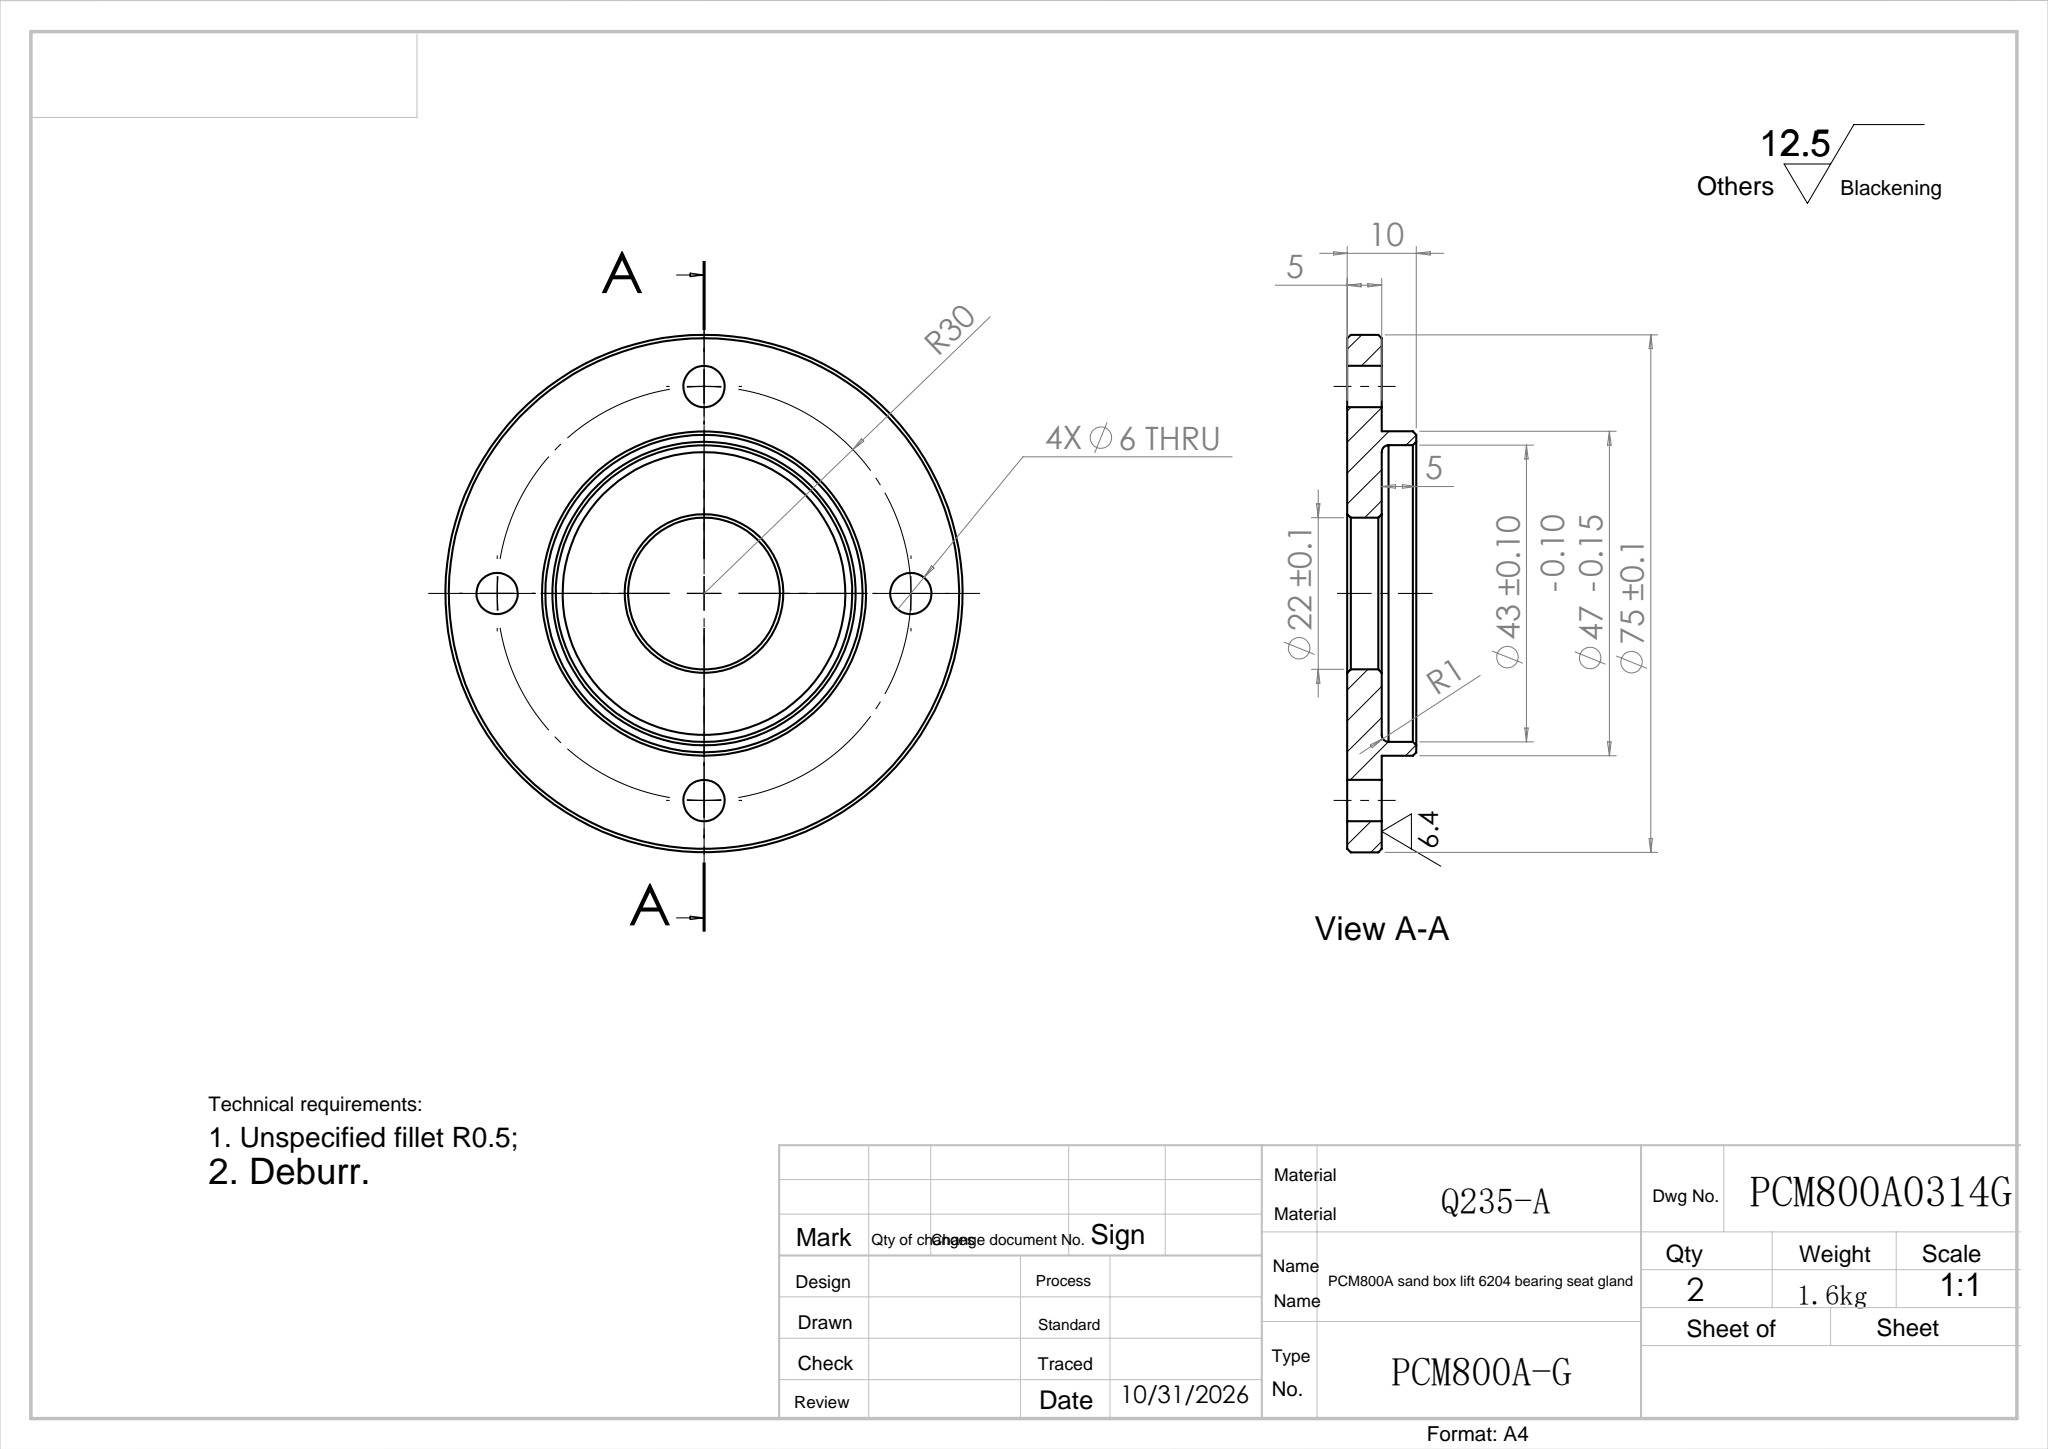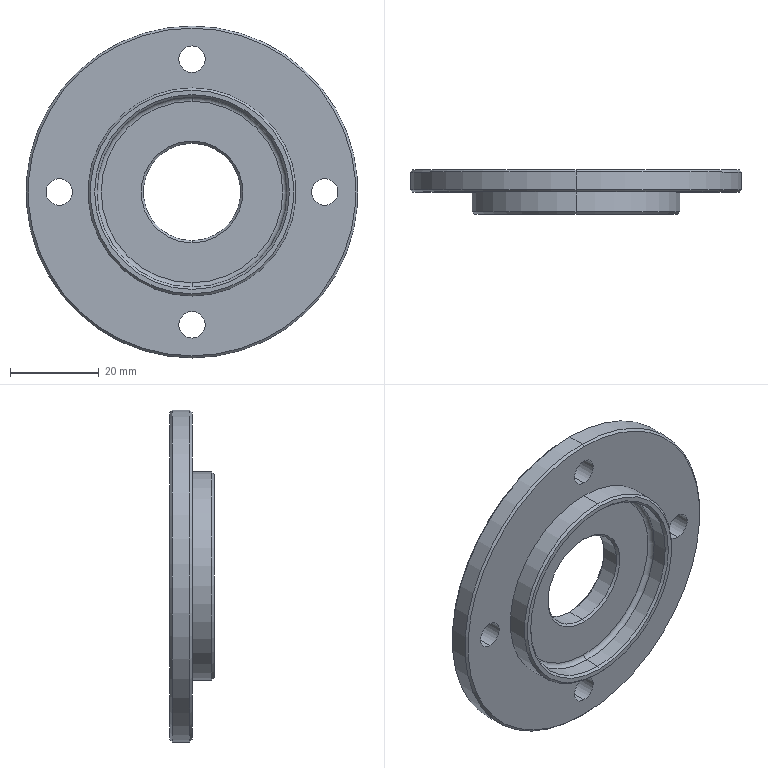Part | SolidWorks | features Chamfer 2, Boss 1, Cut 1, Extrusion 1, Fillet 1 | 1 solid | 34 faces | box 75 x 10 x 75 mm | volume 20954 mm3 | cylinder 16 | cone 12 | plane 4 | torus 2 | commonest cylinder face diameters 6 x8 22 x2 43 x2 47 x2 75 x2
STEP:
#1=CARTESIAN_POINT('',(0.,4.5,-11.));
#2=VERTEX_POINT('',#1);
#3=CARTESIAN_POINT('',(0.,4.5,11.));
#4=VERTEX_POINT('',#3);
#5=CARTESIAN_POINT('',(0.,4.5,0.));
#6=DIRECTION('',(0.,1.,0.));
#7=DIRECTION('',(0.,0.,1.));
#8=AXIS2_PLACEMENT_3D('',#5,#6,#7);
#9=CIRCLE('',#8,11.);
#10=EDGE_CURVE('',#2,#4,#9,.T.);
#11=ORIENTED_EDGE('',*,*,#10,.F.);
#12=CARTESIAN_POINT('',(0.,5.,-11.5));
#13=VERTEX_POINT('',#12);
#14=CARTESIAN_POINT('',(0.,4.5,-11.));
#15=DIRECTION('',(0.,0.7071,-0.7071));
#16=VECTOR('',#15,1000.);
#17=LINE('',#14,#16);
#18=EDGE_CURVE('',#2,#13,#17,.T.);
#19=ORIENTED_EDGE('',*,*,#18,.T.);
#20=CARTESIAN_POINT('',(0.,5.,11.5));
#21=VERTEX_POINT('',#20);
#22=CARTESIAN_POINT('',(0.,5.,0.));
#23=DIRECTION('',(0.,-1.,0.));
#24=DIRECTION('',(0.,0.,1.));
#25=AXIS2_PLACEMENT_3D('',#22,#23,#24);
#26=CIRCLE('',#25,11.5);
#27=EDGE_CURVE('',#21,#13,#26,.T.);
#28=ORIENTED_EDGE('',*,*,#27,.F.);
#29=CARTESIAN_POINT('',(0.,4.5,11.));
#30=DIRECTION('',(0.,0.7071,0.7071));
#31=VECTOR('',#30,1000.);
#32=LINE('',#29,#31);
#33=EDGE_CURVE('',#4,#21,#32,.T.);
#34=ORIENTED_EDGE('',*,*,#33,.F.);
#35=EDGE_LOOP('',(#11,#19,#28,#34));
#36=FACE_OUTER_BOUND('',#35,.T.);
#37=CARTESIAN_POINT('',(0.,4.5,0.));
#38=DIRECTION('',(0.,1.,0.));
#39=DIRECTION('',(0.,0.,1.));
#40=AXIS2_PLACEMENT_3D('',#37,#38,#39);
#41=CONICAL_SURFACE('',#40,11.,0.7854);
#42=ADVANCED_FACE('',(#36),#41,.F.);
#43=CARTESIAN_POINT('',(0.,0.5,11.));
#44=VERTEX_POINT('',#43);
#45=CARTESIAN_POINT('',(0.,0.5,-11.));
#46=VERTEX_POINT('',#45);
#47=CARTESIAN_POINT('',(0.,0.5,0.));
#48=DIRECTION('',(0.,-1.,0.));
#49=DIRECTION('',(0.,0.,1.));
#50=AXIS2_PLACEMENT_3D('',#47,#48,#49);
#51=CIRCLE('',#50,11.);
#52=EDGE_CURVE('',#44,#46,#51,.T.);
#53=ORIENTED_EDGE('',*,*,#52,.F.);
#54=CARTESIAN_POINT('',(0.,0.,11.5));
#55=VERTEX_POINT('',#54);
#56=CARTESIAN_POINT('',(0.,0.,11.5));
#57=DIRECTION('',(0.,-0.7071,0.7071));
#58=VECTOR('',#57,1000.);
#59=LINE('',#56,#58);
#60=EDGE_CURVE('',#44,#55,#59,.T.);
#61=ORIENTED_EDGE('',*,*,#60,.T.);
#62=CARTESIAN_POINT('',(0.,0.,-11.5));
#63=VERTEX_POINT('',#62);
#64=CARTESIAN_POINT('',(0.,0.,0.));
#65=DIRECTION('',(0.,1.,0.));
#66=DIRECTION('',(0.,0.,1.));
#67=AXIS2_PLACEMENT_3D('',#64,#65,#66);
#68=CIRCLE('',#67,11.5);
#69=EDGE_CURVE('',#63,#55,#68,.T.);
#70=ORIENTED_EDGE('',*,*,#69,.F.);
#71=CARTESIAN_POINT('',(0.,0.,-11.5));
#72=DIRECTION('',(0.,-0.7071,-0.7071));
#73=VECTOR('',#72,1000.);
#74=LINE('',#71,#73);
#75=EDGE_CURVE('',#46,#63,#74,.T.);
#76=ORIENTED_EDGE('',*,*,#75,.F.);
#77=EDGE_LOOP('',(#53,#61,#70,#76));
#78=FACE_OUTER_BOUND('',#77,.T.);
#79=CARTESIAN_POINT('',(0.,0.,0.));
#80=DIRECTION('',(0.,-1.,0.));
#81=DIRECTION('',(0.,0.,-1.));
#82=AXIS2_PLACEMENT_3D('',#79,#80,#81);
#83=CONICAL_SURFACE('',#82,11.5,0.7854);
#84=ADVANCED_FACE('',(#78),#83,.F.);
#85=CARTESIAN_POINT('',(0.,-1.,-21.5));
#86=VERTEX_POINT('',#85);
#87=CARTESIAN_POINT('',(0.,-1.,21.5));
#88=VERTEX_POINT('',#87);
#89=CARTESIAN_POINT('',(0.,-1.,0.));
#90=DIRECTION('',(0.,1.,0.));
#91=DIRECTION('',(0.,0.,1.));
#92=AXIS2_PLACEMENT_3D('',#89,#90,#91);
#93=CIRCLE('',#92,21.5);
#94=EDGE_CURVE('',#86,#88,#93,.T.);
#95=ORIENTED_EDGE('',*,*,#94,.F.);
#96=CARTESIAN_POINT('',(0.,0.,-20.5));
#97=VERTEX_POINT('',#96);
#98=CARTESIAN_POINT('',(0.,-1.,-20.5));
#99=DIRECTION('',(1.,0.,0.));
#100=DIRECTION('',(0.,0.,-1.));
#101=AXIS2_PLACEMENT_3D('',#98,#99,#100);
#102=CIRCLE('',#101,1.);
#103=EDGE_CURVE('',#86,#97,#102,.T.);
#104=ORIENTED_EDGE('',*,*,#103,.T.);
#105=CARTESIAN_POINT('',(0.,0.,20.5));
#106=VERTEX_POINT('',#105);
#107=CARTESIAN_POINT('',(0.,0.,0.));
#108=DIRECTION('',(0.,-1.,0.));
#109=DIRECTION('',(0.,0.,1.));
#110=AXIS2_PLACEMENT_3D('',#107,#108,#109);
#111=CIRCLE('',#110,20.5);
#112=EDGE_CURVE('',#106,#97,#111,.T.);
#113=ORIENTED_EDGE('',*,*,#112,.F.);
#114=CARTESIAN_POINT('',(0.,-1.,20.5));
#115=DIRECTION('',(-1.,0.,0.));
#116=DIRECTION('',(0.,0.,1.));
#117=AXIS2_PLACEMENT_3D('',#114,#115,#116);
#118=CIRCLE('',#117,1.);
#119=EDGE_CURVE('',#88,#106,#118,.T.);
#120=ORIENTED_EDGE('',*,*,#119,.F.);
#121=EDGE_LOOP('',(#95,#104,#113,#120));
#122=FACE_OUTER_BOUND('',#121,.T.);
#123=CARTESIAN_POINT('',(0.,-1.,0.));
#124=DIRECTION('',(0.,1.,0.));
#125=DIRECTION('',(0.,0.,1.));
#126=AXIS2_PLACEMENT_3D('',#123,#124,#125);
#127=TOROIDAL_SURFACE('',#126,20.5,1.);
#128=ADVANCED_FACE('',(#122),#127,.F.);
#129=CARTESIAN_POINT('',(0.,-5.,-23.));
#130=VERTEX_POINT('',#129);
#131=CARTESIAN_POINT('',(0.,-5.,23.));
#132=VERTEX_POINT('',#131);
#133=CARTESIAN_POINT('',(0.,-5.,0.));
#134=DIRECTION('',(0.,-1.,0.));
#135=DIRECTION('',(0.,0.,-1.));
#136=AXIS2_PLACEMENT_3D('',#133,#134,#135);
#137=CIRCLE('',#136,23.);
#138=EDGE_CURVE('',#130,#132,#137,.T.);
#139=ORIENTED_EDGE('',*,*,#138,.F.);
#140=CARTESIAN_POINT('',(0.,-4.5,-23.5));
#141=VERTEX_POINT('',#140);
#142=CARTESIAN_POINT('',(0.,-5.,-23.));
#143=DIRECTION('',(0.,0.7071,-0.7071));
#144=VECTOR('',#143,1000.);
#145=LINE('',#142,#144);
#146=EDGE_CURVE('',#130,#141,#145,.T.);
#147=ORIENTED_EDGE('',*,*,#146,.T.);
#148=CARTESIAN_POINT('',(0.,-4.5,23.5));
#149=VERTEX_POINT('',#148);
#150=CARTESIAN_POINT('',(0.,-4.5,0.));
#151=DIRECTION('',(0.,1.,0.));
#152=DIRECTION('',(0.,0.,-1.));
#153=AXIS2_PLACEMENT_3D('',#150,#151,#152);
#154=CIRCLE('',#153,23.5);
#155=EDGE_CURVE('',#149,#141,#154,.T.);
#156=ORIENTED_EDGE('',*,*,#155,.F.);
#157=CARTESIAN_POINT('',(0.,-5.,23.));
#158=DIRECTION('',(0.,0.7071,0.7071));
#159=VECTOR('',#158,1000.);
#160=LINE('',#157,#159);
#161=EDGE_CURVE('',#132,#149,#160,.T.);
#162=ORIENTED_EDGE('',*,*,#161,.F.);
#163=EDGE_LOOP('',(#139,#147,#156,#162));
#164=FACE_OUTER_BOUND('',#163,.T.);
#165=CARTESIAN_POINT('',(0.,-5.,0.));
#166=DIRECTION('',(0.,1.,0.));
#167=DIRECTION('',(0.,0.,1.));
#168=AXIS2_PLACEMENT_3D('',#165,#166,#167);
#169=CONICAL_SURFACE('',#168,23.,0.7854);
#170=ADVANCED_FACE('',(#164),#169,.T.);
#171=CARTESIAN_POINT('',(0.,-4.5,21.5));
#172=VERTEX_POINT('',#171);
#173=CARTESIAN_POINT('',(0.,-4.5,-21.5));
#174=VERTEX_POINT('',#173);
#175=CARTESIAN_POINT('',(0.,-4.5,0.));
#176=DIRECTION('',(0.,-1.,0.));
#177=DIRECTION('',(0.,0.,-1.));
#178=AXIS2_PLACEMENT_3D('',#175,#176,#177);
#179=CIRCLE('',#178,21.5);
#180=EDGE_CURVE('',#172,#174,#179,.T.);
#181=ORIENTED_EDGE('',*,*,#180,.F.);
#182=CARTESIAN_POINT('',(0.,-5.,22.));
#183=VERTEX_POINT('',#182);
#184=CARTESIAN_POINT('',(0.,-4.5,21.5));
#185=DIRECTION('',(0.,-0.7071,0.7071));
#186=VECTOR('',#185,1000.);
#187=LINE('',#184,#186);
#188=EDGE_CURVE('',#172,#183,#187,.T.);
#189=ORIENTED_EDGE('',*,*,#188,.T.);
#190=CARTESIAN_POINT('',(0.,-5.,-22.));
#191=VERTEX_POINT('',#190);
#192=CARTESIAN_POINT('',(0.,-5.,0.));
#193=DIRECTION('',(0.,1.,0.));
#194=DIRECTION('',(0.,0.,-1.));
#195=AXIS2_PLACEMENT_3D('',#192,#193,#194);
#196=CIRCLE('',#195,22.);
#197=EDGE_CURVE('',#191,#183,#196,.T.);
#198=ORIENTED_EDGE('',*,*,#197,.F.);
#199=CARTESIAN_POINT('',(0.,-4.5,-21.5));
#200=DIRECTION('',(0.,-0.7071,-0.7071));
#201=VECTOR('',#200,1000.);
#202=LINE('',#199,#201);
#203=EDGE_CURVE('',#174,#191,#202,.T.);
#204=ORIENTED_EDGE('',*,*,#203,.F.);
#205=EDGE_LOOP('',(#181,#189,#198,#204));
#206=FACE_OUTER_BOUND('',#205,.T.);
#207=CARTESIAN_POINT('',(0.,-4.5,0.));
#208=DIRECTION('',(0.,-1.,0.));
#209=DIRECTION('',(0.,0.,-1.));
#210=AXIS2_PLACEMENT_3D('',#207,#208,#209);
#211=CONICAL_SURFACE('',#210,21.5,0.7854);
#212=ADVANCED_FACE('',(#206),#211,.F.);
#213=CARTESIAN_POINT('',(0.,0.,-37.));
#214=VERTEX_POINT('',#213);
#215=CARTESIAN_POINT('',(0.,0.,37.));
#216=VERTEX_POINT('',#215);
#217=CARTESIAN_POINT('',(0.,0.,0.));
#218=DIRECTION('',(0.,-1.,0.));
#219=DIRECTION('',(0.,0.,1.));
#220=AXIS2_PLACEMENT_3D('',#217,#218,#219);
#221=CIRCLE('',#220,37.);
#222=EDGE_CURVE('',#214,#216,#221,.T.);
#223=ORIENTED_EDGE('',*,*,#222,.F.);
#224=CARTESIAN_POINT('',(0.,0.5,-37.5));
#225=VERTEX_POINT('',#224);
#226=CARTESIAN_POINT('',(0.,0.5,-37.5));
#227=DIRECTION('',(0.,0.7071,-0.7071));
#228=VECTOR('',#227,1000.);
#229=LINE('',#226,#228);
#230=EDGE_CURVE('',#214,#225,#229,.T.);
#231=ORIENTED_EDGE('',*,*,#230,.T.);
#232=CARTESIAN_POINT('',(0.,0.5,37.5));
#233=VERTEX_POINT('',#232);
#234=CARTESIAN_POINT('',(0.,0.5,0.));
#235=DIRECTION('',(0.,1.,0.));
#236=DIRECTION('',(0.,0.,1.));
#237=AXIS2_PLACEMENT_3D('',#234,#235,#236);
#238=CIRCLE('',#237,37.5);
#239=EDGE_CURVE('',#233,#225,#238,.T.);
#240=ORIENTED_EDGE('',*,*,#239,.F.);
#241=CARTESIAN_POINT('',(0.,0.5,37.5));
#242=DIRECTION('',(0.,0.7071,0.7071));
#243=VECTOR('',#242,1000.);
#244=LINE('',#241,#243);
#245=EDGE_CURVE('',#216,#233,#244,.T.);
#246=ORIENTED_EDGE('',*,*,#245,.F.);
#247=EDGE_LOOP('',(#223,#231,#240,#246));
#248=FACE_OUTER_BOUND('',#247,.T.);
#249=CARTESIAN_POINT('',(0.,0.5,0.));
#250=DIRECTION('',(0.,1.,0.));
#251=DIRECTION('',(0.,0.,1.));
#252=AXIS2_PLACEMENT_3D('',#249,#250,#251);
#253=CONICAL_SURFACE('',#252,37.5,0.7854);
#254=ADVANCED_FACE('',(#248),#253,.T.);
#255=CARTESIAN_POINT('',(0.,5.,37.));
#256=VERTEX_POINT('',#255);
#257=CARTESIAN_POINT('',(0.,5.,-37.));
#258=VERTEX_POINT('',#257);
#259=CARTESIAN_POINT('',(0.,5.,0.));
#260=DIRECTION('',(0.,1.,0.));
#261=DIRECTION('',(0.,0.,1.));
#262=AXIS2_PLACEMENT_3D('',#259,#260,#261);
#263=CIRCLE('',#262,37.);
#264=EDGE_CURVE('',#256,#258,#263,.T.);
#265=ORIENTED_EDGE('',*,*,#264,.F.);
#266=CARTESIAN_POINT('',(0.,4.5,37.5));
#267=VERTEX_POINT('',#266);
#268=CARTESIAN_POINT('',(0.,5.,37.));
#269=DIRECTION('',(0.,-0.7071,0.7071));
#270=VECTOR('',#269,1000.);
#271=LINE('',#268,#270);
#272=EDGE_CURVE('',#256,#267,#271,.T.);
#273=ORIENTED_EDGE('',*,*,#272,.T.);
#274=CARTESIAN_POINT('',(0.,4.5,-37.5));
#275=VERTEX_POINT('',#274);
#276=CARTESIAN_POINT('',(0.,4.5,0.));
#277=DIRECTION('',(0.,-1.,0.));
#278=DIRECTION('',(0.,0.,1.));
#279=AXIS2_PLACEMENT_3D('',#276,#277,#278);
#280=CIRCLE('',#279,37.5);
#281=EDGE_CURVE('',#275,#267,#280,.T.);
#282=ORIENTED_EDGE('',*,*,#281,.F.);
#283=CARTESIAN_POINT('',(0.,5.,-37.));
#284=DIRECTION('',(0.,-0.7071,-0.7071));
#285=VECTOR('',#284,1000.);
#286=LINE('',#283,#285);
#287=EDGE_CURVE('',#258,#275,#286,.T.);
#288=ORIENTED_EDGE('',*,*,#287,.F.);
#289=EDGE_LOOP('',(#265,#273,#282,#288));
#290=FACE_OUTER_BOUND('',#289,.T.);
#291=CARTESIAN_POINT('',(0.,5.,0.));
#292=DIRECTION('',(0.,-1.,0.));
#293=DIRECTION('',(0.,0.,-1.));
#294=AXIS2_PLACEMENT_3D('',#291,#292,#293);
#295=CONICAL_SURFACE('',#294,37.,0.7854);
#296=ADVANCED_FACE('',(#290),#295,.T.);
#297=CARTESIAN_POINT('',(0.,0.,-33.));
#298=VERTEX_POINT('',#297);
#299=CARTESIAN_POINT('',(0.,0.,-27.));
#300=VERTEX_POINT('',#299);
#301=CARTESIAN_POINT('',(0.,0.,-30.));
#302=DIRECTION('',(0.,1.,0.));
#303=DIRECTION('',(0.,0.,1.));
#304=AXIS2_PLACEMENT_3D('',#301,#302,#303);
#305=CIRCLE('',#304,3.);
#306=EDGE_CURVE('',#298,#300,#305,.T.);
#307=ORIENTED_EDGE('',*,*,#306,.F.);
#308=CARTESIAN_POINT('',(0.,5.,-33.));
#309=VERTEX_POINT('',#308);
#310=CARTESIAN_POINT('',(0.,-5.,-33.));
#311=DIRECTION('',(0.,1.,0.));
#312=VECTOR('',#311,1000.);
#313=LINE('',#310,#312);
#314=EDGE_CURVE('',#298,#309,#313,.T.);
#315=ORIENTED_EDGE('',*,*,#314,.T.);
#316=CARTESIAN_POINT('',(0.,5.,-27.));
#317=VERTEX_POINT('',#316);
#318=CARTESIAN_POINT('',(0.,5.,-30.));
#319=DIRECTION('',(0.,1.,0.));
#320=DIRECTION('',(0.,0.,1.));
#321=AXIS2_PLACEMENT_3D('',#318,#319,#320);
#322=CIRCLE('',#321,3.);
#323=EDGE_CURVE('',#309,#317,#322,.T.);
#324=ORIENTED_EDGE('',*,*,#323,.T.);
#325=CARTESIAN_POINT('',(0.,-5.,-27.));
#326=DIRECTION('',(0.,1.,0.));
#327=VECTOR('',#326,1000.);
#328=LINE('',#325,#327);
#329=EDGE_CURVE('',#300,#317,#328,.T.);
#330=ORIENTED_EDGE('',*,*,#329,.F.);
#331=EDGE_LOOP('',(#307,#315,#324,#330));
#332=FACE_OUTER_BOUND('',#331,.T.);
#333=CARTESIAN_POINT('',(0.,-5.,-30.));
#334=DIRECTION('',(0.,1.,0.));
#335=DIRECTION('',(0.,0.,1.));
#336=AXIS2_PLACEMENT_3D('',#333,#334,#335);
#337=CYLINDRICAL_SURFACE('',#336,3.);
#338=ADVANCED_FACE('',(#332),#337,.F.);
#339=CARTESIAN_POINT('',(-30.,0.,-3.));
#340=VERTEX_POINT('',#339);
#341=CARTESIAN_POINT('',(-30.,0.,3.));
#342=VERTEX_POINT('',#341);
#343=CARTESIAN_POINT('',(-30.,0.,0.));
#344=DIRECTION('',(0.,1.,0.));
#345=DIRECTION('',(0.,0.,1.));
#346=AXIS2_PLACEMENT_3D('',#343,#344,#345);
#347=CIRCLE('',#346,3.);
#348=EDGE_CURVE('',#340,#342,#347,.T.);
#349=ORIENTED_EDGE('',*,*,#348,.F.);
#350=CARTESIAN_POINT('',(-30.,5.,-3.));
#351=VERTEX_POINT('',#350);
#352=CARTESIAN_POINT('',(-30.,-5.,-3.));
#353=DIRECTION('',(0.,1.,0.));
#354=VECTOR('',#353,1000.);
#355=LINE('',#352,#354);
#356=EDGE_CURVE('',#340,#351,#355,.T.);
#357=ORIENTED_EDGE('',*,*,#356,.T.);
#358=CARTESIAN_POINT('',(-30.,5.,3.));
#359=VERTEX_POINT('',#358);
#360=CARTESIAN_POINT('',(-30.,5.,0.));
#361=DIRECTION('',(0.,1.,0.));
#362=DIRECTION('',(0.,0.,1.));
#363=AXIS2_PLACEMENT_3D('',#360,#361,#362);
#364=CIRCLE('',#363,3.);
#365=EDGE_CURVE('',#351,#359,#364,.T.);
#366=ORIENTED_EDGE('',*,*,#365,.T.);
#367=CARTESIAN_POINT('',(-30.,-5.,3.));
#368=DIRECTION('',(0.,1.,0.));
#369=VECTOR('',#368,1000.);
#370=LINE('',#367,#369);
#371=EDGE_CURVE('',#342,#359,#370,.T.);
#372=ORIENTED_EDGE('',*,*,#371,.F.);
#373=EDGE_LOOP('',(#349,#357,#366,#372));
#374=FACE_OUTER_BOUND('',#373,.T.);
#375=CARTESIAN_POINT('',(-30.,-5.,0.));
#376=DIRECTION('',(0.,1.,0.));
#377=DIRECTION('',(0.,0.,1.));
#378=AXIS2_PLACEMENT_3D('',#375,#376,#377);
#379=CYLINDRICAL_SURFACE('',#378,3.);
#380=ADVANCED_FACE('',(#374),#379,.F.);
#381=CARTESIAN_POINT('',(0.,0.,27.));
#382=VERTEX_POINT('',#381);
#383=CARTESIAN_POINT('',(0.,0.,33.));
#384=VERTEX_POINT('',#383);
#385=CARTESIAN_POINT('',(0.,0.,30.));
#386=DIRECTION('',(0.,1.,0.));
#387=DIRECTION('',(0.,0.,1.));
#388=AXIS2_PLACEMENT_3D('',#385,#386,#387);
#389=CIRCLE('',#388,3.);
#390=EDGE_CURVE('',#382,#384,#389,.T.);
#391=ORIENTED_EDGE('',*,*,#390,.F.);
#392=CARTESIAN_POINT('',(0.,5.,27.));
#393=VERTEX_POINT('',#392);
#394=CARTESIAN_POINT('',(0.,-5.,27.));
#395=DIRECTION('',(0.,1.,0.));
#396=VECTOR('',#395,1000.);
#397=LINE('',#394,#396);
#398=EDGE_CURVE('',#382,#393,#397,.T.);
#399=ORIENTED_EDGE('',*,*,#398,.T.);
#400=CARTESIAN_POINT('',(0.,5.,33.));
#401=VERTEX_POINT('',#400);
#402=CARTESIAN_POINT('',(0.,5.,30.));
#403=DIRECTION('',(0.,1.,0.));
#404=DIRECTION('',(0.,0.,1.));
#405=AXIS2_PLACEMENT_3D('',#402,#403,#404);
#406=CIRCLE('',#405,3.);
#407=EDGE_CURVE('',#393,#401,#406,.T.);
#408=ORIENTED_EDGE('',*,*,#407,.T.);
#409=CARTESIAN_POINT('',(0.,-5.,33.));
#410=DIRECTION('',(0.,1.,0.));
#411=VECTOR('',#410,1000.);
#412=LINE('',#409,#411);
#413=EDGE_CURVE('',#384,#401,#412,.T.);
#414=ORIENTED_EDGE('',*,*,#413,.F.);
#415=EDGE_LOOP('',(#391,#399,#408,#414));
#416=FACE_OUTER_BOUND('',#415,.T.);
#417=CARTESIAN_POINT('',(0.,-5.,30.));
#418=DIRECTION('',(0.,1.,0.));
#419=DIRECTION('',(0.,0.,1.));
#420=AXIS2_PLACEMENT_3D('',#417,#418,#419);
#421=CYLINDRICAL_SURFACE('',#420,3.);
#422=ADVANCED_FACE('',(#416),#421,.F.);
#423=CARTESIAN_POINT('',(30.,0.,-3.));
#424=VERTEX_POINT('',#423);
#425=CARTESIAN_POINT('',(30.,0.,3.));
#426=VERTEX_POINT('',#425);
#427=CARTESIAN_POINT('',(30.,0.,0.));
#428=DIRECTION('',(0.,1.,0.));
#429=DIRECTION('',(0.,0.,1.));
#430=AXIS2_PLACEMENT_3D('',#427,#428,#429);
#431=CIRCLE('',#430,3.);
#432=EDGE_CURVE('',#424,#426,#431,.T.);
#433=ORIENTED_EDGE('',*,*,#432,.F.);
#434=CARTESIAN_POINT('',(30.,5.,-3.));
#435=VERTEX_POINT('',#434);
#436=CARTESIAN_POINT('',(30.,-5.,-3.));
#437=DIRECTION('',(0.,1.,0.));
#438=VECTOR('',#437,1000.);
#439=LINE('',#436,#438);
#440=EDGE_CURVE('',#424,#435,#439,.T.);
#441=ORIENTED_EDGE('',*,*,#440,.T.);
#442=CARTESIAN_POINT('',(30.,5.,3.));
#443=VERTEX_POINT('',#442);
#444=CARTESIAN_POINT('',(30.,5.,0.));
#445=DIRECTION('',(0.,1.,0.));
#446=DIRECTION('',(0.,0.,1.));
#447=AXIS2_PLACEMENT_3D('',#444,#445,#446);
#448=CIRCLE('',#447,3.);
#449=EDGE_CURVE('',#435,#443,#448,.T.);
#450=ORIENTED_EDGE('',*,*,#449,.T.);
#451=CARTESIAN_POINT('',(30.,-5.,3.));
#452=DIRECTION('',(0.,1.,0.));
#453=VECTOR('',#452,1000.);
#454=LINE('',#451,#453);
#455=EDGE_CURVE('',#426,#443,#454,.T.);
#456=ORIENTED_EDGE('',*,*,#455,.F.);
#457=EDGE_LOOP('',(#433,#441,#450,#456));
#458=FACE_OUTER_BOUND('',#457,.T.);
#459=CARTESIAN_POINT('',(30.,-5.,0.));
#460=DIRECTION('',(0.,1.,0.));
#461=DIRECTION('',(0.,0.,1.));
#462=AXIS2_PLACEMENT_3D('',#459,#460,#461);
#463=CYLINDRICAL_SURFACE('',#462,3.);
#464=ADVANCED_FACE('',(#458),#463,.F.);
#465=ORIENTED_EDGE('',*,*,#180,.T.);
#466=CARTESIAN_POINT('',(0.,-5.,-21.5));
#467=DIRECTION('',(0.,1.,0.));
#468=VECTOR('',#467,1000.);
#469=LINE('',#466,#468);
#470=EDGE_CURVE('',#174,#86,#469,.T.);
#471=ORIENTED_EDGE('',*,*,#470,.T.);
#472=ORIENTED_EDGE('',*,*,#94,.T.);
#473=CARTESIAN_POINT('',(0.,-5.,21.5));
#474=DIRECTION('',(0.,1.,0.));
#475=VECTOR('',#474,1000.);
#476=LINE('',#473,#475);
#477=EDGE_CURVE('',#172,#88,#476,.T.);
#478=ORIENTED_EDGE('',*,*,#477,.F.);
#479=EDGE_LOOP('',(#465,#471,#472,#478));
#480=FACE_OUTER_BOUND('',#479,.T.);
#481=CARTESIAN_POINT('',(0.,-5.,0.));
#482=DIRECTION('',(0.,1.,0.));
#483=DIRECTION('',(0.,0.,1.));
#484=AXIS2_PLACEMENT_3D('',#481,#482,#483);
#485=CYLINDRICAL_SURFACE('',#484,21.5);
#486=ADVANCED_FACE('',(#480),#485,.F.);
#487=ORIENTED_EDGE('',*,*,#155,.T.);
#488=CARTESIAN_POINT('',(0.,0.,-23.5));
#489=VERTEX_POINT('',#488);
#490=CARTESIAN_POINT('',(0.,-5.,-23.5));
#491=DIRECTION('',(0.,1.,0.));
#492=VECTOR('',#491,1000.);
#493=LINE('',#490,#492);
#494=EDGE_CURVE('',#141,#489,#493,.T.);
#495=ORIENTED_EDGE('',*,*,#494,.T.);
#496=CARTESIAN_POINT('',(0.,0.,23.5));
#497=VERTEX_POINT('',#496);
#498=CARTESIAN_POINT('',(0.,0.,0.));
#499=DIRECTION('',(0.,-1.,0.));
#500=DIRECTION('',(0.,0.,1.));
#501=AXIS2_PLACEMENT_3D('',#498,#499,#500);
#502=CIRCLE('',#501,23.5);
#503=EDGE_CURVE('',#489,#497,#502,.T.);
#504=ORIENTED_EDGE('',*,*,#503,.T.);
#505=CARTESIAN_POINT('',(0.,-5.,23.5));
#506=DIRECTION('',(0.,1.,0.));
#507=VECTOR('',#506,1000.);
#508=LINE('',#505,#507);
#509=EDGE_CURVE('',#149,#497,#508,.T.);
#510=ORIENTED_EDGE('',*,*,#509,.F.);
#511=EDGE_LOOP('',(#487,#495,#504,#510));
#512=FACE_OUTER_BOUND('',#511,.T.);
#513=CARTESIAN_POINT('',(0.,-5.,0.));
#514=DIRECTION('',(0.,1.,0.));
#515=DIRECTION('',(0.,0.,1.));
#516=AXIS2_PLACEMENT_3D('',#513,#514,#515);
#517=CYLINDRICAL_SURFACE('',#516,23.5);
#518=ADVANCED_FACE('',(#512),#517,.T.);
#519=ORIENTED_EDGE('',*,*,#10,.T.);
#520=CARTESIAN_POINT('',(0.,5.,11.));
#521=DIRECTION('',(0.,-1.,0.));
#522=VECTOR('',#521,1000.);
#523=LINE('',#520,#522);
#524=EDGE_CURVE('',#4,#44,#523,.T.);
#525=ORIENTED_EDGE('',*,*,#524,.T.);
#526=ORIENTED_EDGE('',*,*,#52,.T.);
#527=CARTESIAN_POINT('',(0.,5.,-11.));
#528=DIRECTION('',(0.,-1.,0.));
#529=VECTOR('',#528,1000.);
#530=LINE('',#527,#529);
#531=EDGE_CURVE('',#2,#46,#530,.T.);
#532=ORIENTED_EDGE('',*,*,#531,.F.);
#533=EDGE_LOOP('',(#519,#525,#526,#532));
#534=FACE_OUTER_BOUND('',#533,.T.);
#535=CARTESIAN_POINT('',(0.,5.,0.));
#536=DIRECTION('',(0.,-1.,0.));
#537=DIRECTION('',(0.,0.,-1.));
#538=AXIS2_PLACEMENT_3D('',#535,#536,#537);
#539=CYLINDRICAL_SURFACE('',#538,11.);
#540=ADVANCED_FACE('',(#534),#539,.F.);
#541=ORIENTED_EDGE('',*,*,#281,.T.);
#542=CARTESIAN_POINT('',(0.,5.,37.5));
#543=DIRECTION('',(0.,-1.,0.));
#544=VECTOR('',#543,1000.);
#545=LINE('',#542,#544);
#546=EDGE_CURVE('',#267,#233,#545,.T.);
#547=ORIENTED_EDGE('',*,*,#546,.T.);
#548=ORIENTED_EDGE('',*,*,#239,.T.);
#549=CARTESIAN_POINT('',(0.,5.,-37.5));
#550=DIRECTION('',(0.,-1.,0.));
#551=VECTOR('',#550,1000.);
#552=LINE('',#549,#551);
#553=EDGE_CURVE('',#275,#225,#552,.T.);
#554=ORIENTED_EDGE('',*,*,#553,.F.);
#555=EDGE_LOOP('',(#541,#547,#548,#554));
#556=FACE_OUTER_BOUND('',#555,.T.);
#557=CARTESIAN_POINT('',(0.,5.,0.));
#558=DIRECTION('',(0.,-1.,0.));
#559=DIRECTION('',(0.,0.,-1.));
#560=AXIS2_PLACEMENT_3D('',#557,#558,#559);
#561=CYLINDRICAL_SURFACE('',#560,37.5);
#562=ADVANCED_FACE('',(#556),#561,.T.);
#563=CARTESIAN_POINT('',(0.,0.,0.));
#564=DIRECTION('',(0.,-1.,0.));
#565=DIRECTION('',(0.,0.,1.));
#566=AXIS2_PLACEMENT_3D('',#563,#564,#565);
#567=CIRCLE('',#566,37.);
#568=EDGE_CURVE('',#216,#214,#567,.T.);
#569=ORIENTED_EDGE('',*,*,#568,.T.);
#570=ORIENTED_EDGE('',*,*,#222,.T.);
#571=EDGE_LOOP('',(#569,#570));
#572=FACE_OUTER_BOUND('',#571,.T.);
#573=CARTESIAN_POINT('',(0.,0.,-30.));
#574=DIRECTION('',(0.,1.,0.));
#575=DIRECTION('',(0.,0.,1.));
#576=AXIS2_PLACEMENT_3D('',#573,#574,#575);
#577=CIRCLE('',#576,3.);
#578=EDGE_CURVE('',#300,#298,#577,.T.);
#579=ORIENTED_EDGE('',*,*,#578,.T.);
#580=ORIENTED_EDGE('',*,*,#306,.T.);
#581=EDGE_LOOP('',(#579,#580));
#582=FACE_BOUND('',#581,.T.);
#583=CARTESIAN_POINT('',(-30.,0.,0.));
#584=DIRECTION('',(0.,1.,0.));
#585=DIRECTION('',(0.,0.,1.));
#586=AXIS2_PLACEMENT_3D('',#583,#584,#585);
#587=CIRCLE('',#586,3.);
#588=EDGE_CURVE('',#342,#340,#587,.T.);
#589=ORIENTED_EDGE('',*,*,#588,.T.);
#590=ORIENTED_EDGE('',*,*,#348,.T.);
#591=EDGE_LOOP('',(#589,#590));
#592=FACE_BOUND('',#591,.T.);
#593=CARTESIAN_POINT('',(0.,0.,30.));
#594=DIRECTION('',(0.,1.,0.));
#595=DIRECTION('',(0.,0.,1.));
#596=AXIS2_PLACEMENT_3D('',#593,#594,#595);
#597=CIRCLE('',#596,3.);
#598=EDGE_CURVE('',#384,#382,#597,.T.);
#599=ORIENTED_EDGE('',*,*,#598,.T.);
#600=ORIENTED_EDGE('',*,*,#390,.T.);
#601=EDGE_LOOP('',(#599,#600));
#602=FACE_BOUND('',#601,.T.);
#603=CARTESIAN_POINT('',(30.,0.,0.));
#604=DIRECTION('',(0.,1.,0.));
#605=DIRECTION('',(0.,0.,1.));
#606=AXIS2_PLACEMENT_3D('',#603,#604,#605);
#607=CIRCLE('',#606,3.);
#608=EDGE_CURVE('',#426,#424,#607,.T.);
#609=ORIENTED_EDGE('',*,*,#608,.T.);
#610=ORIENTED_EDGE('',*,*,#432,.T.);
#611=EDGE_LOOP('',(#609,#610));
#612=FACE_BOUND('',#611,.T.);
#613=CARTESIAN_POINT('',(0.,0.,0.));
#614=DIRECTION('',(0.,-1.,0.));
#615=DIRECTION('',(0.,0.,1.));
#616=AXIS2_PLACEMENT_3D('',#613,#614,#615);
#617=CIRCLE('',#616,23.5);
#618=EDGE_CURVE('',#497,#489,#617,.T.);
#619=ORIENTED_EDGE('',*,*,#618,.F.);
#620=ORIENTED_EDGE('',*,*,#503,.F.);
#621=EDGE_LOOP('',(#619,#620));
#622=FACE_BOUND('',#621,.T.);
#623=CARTESIAN_POINT('',(0.,0.,0.));
#624=DIRECTION('',(0.,1.,0.));
#625=DIRECTION('',(0.,0.,1.));
#626=AXIS2_PLACEMENT_3D('',#623,#624,#625);
#627=PLANE('',#626);
#628=ADVANCED_FACE('',(#572,#582,#592,#602,#612,#622),#627,.F.);
#629=ORIENTED_EDGE('',*,*,#27,.T.);
#630=CARTESIAN_POINT('',(0.,5.,0.));
#631=DIRECTION('',(0.,-1.,0.));
#632=DIRECTION('',(0.,0.,1.));
#633=AXIS2_PLACEMENT_3D('',#630,#631,#632);
#634=CIRCLE('',#633,11.5);
#635=EDGE_CURVE('',#13,#21,#634,.T.);
#636=ORIENTED_EDGE('',*,*,#635,.T.);
#637=EDGE_LOOP('',(#629,#636));
#638=FACE_BOUND('',#637,.T.);
#639=CARTESIAN_POINT('',(0.,5.,0.));
#640=DIRECTION('',(0.,1.,0.));
#641=DIRECTION('',(0.,0.,1.));
#642=AXIS2_PLACEMENT_3D('',#639,#640,#641);
#643=CIRCLE('',#642,37.);
#644=EDGE_CURVE('',#258,#256,#643,.T.);
#645=ORIENTED_EDGE('',*,*,#644,.T.);
#646=ORIENTED_EDGE('',*,*,#264,.T.);
#647=EDGE_LOOP('',(#645,#646));
#648=FACE_OUTER_BOUND('',#647,.T.);
#649=CARTESIAN_POINT('',(0.,5.,-30.));
#650=DIRECTION('',(0.,1.,0.));
#651=DIRECTION('',(0.,0.,1.));
#652=AXIS2_PLACEMENT_3D('',#649,#650,#651);
#653=CIRCLE('',#652,3.);
#654=EDGE_CURVE('',#317,#309,#653,.T.);
#655=ORIENTED_EDGE('',*,*,#654,.F.);
#656=ORIENTED_EDGE('',*,*,#323,.F.);
#657=EDGE_LOOP('',(#655,#656));
#658=FACE_BOUND('',#657,.T.);
#659=CARTESIAN_POINT('',(-30.,5.,0.));
#660=DIRECTION('',(0.,1.,0.));
#661=DIRECTION('',(0.,0.,1.));
#662=AXIS2_PLACEMENT_3D('',#659,#660,#661);
#663=CIRCLE('',#662,3.);
#664=EDGE_CURVE('',#359,#351,#663,.T.);
#665=ORIENTED_EDGE('',*,*,#664,.F.);
#666=ORIENTED_EDGE('',*,*,#365,.F.);
#667=EDGE_LOOP('',(#665,#666));
#668=FACE_BOUND('',#667,.T.);
#669=CARTESIAN_POINT('',(0.,5.,30.));
#670=DIRECTION('',(0.,1.,0.));
#671=DIRECTION('',(0.,0.,1.));
#672=AXIS2_PLACEMENT_3D('',#669,#670,#671);
#673=CIRCLE('',#672,3.);
#674=EDGE_CURVE('',#401,#393,#673,.T.);
#675=ORIENTED_EDGE('',*,*,#674,.F.);
#676=ORIENTED_EDGE('',*,*,#407,.F.);
#677=EDGE_LOOP('',(#675,#676));
#678=FACE_BOUND('',#677,.T.);
#679=CARTESIAN_POINT('',(30.,5.,0.));
#680=DIRECTION('',(0.,1.,0.));
#681=DIRECTION('',(0.,0.,1.));
#682=AXIS2_PLACEMENT_3D('',#679,#680,#681);
#683=CIRCLE('',#682,3.);
#684=EDGE_CURVE('',#443,#435,#683,.T.);
#685=ORIENTED_EDGE('',*,*,#684,.F.);
#686=ORIENTED_EDGE('',*,*,#449,.F.);
#687=EDGE_LOOP('',(#685,#686));
#688=FACE_BOUND('',#687,.T.);
#689=CARTESIAN_POINT('',(0.,5.,0.));
#690=DIRECTION('',(0.,1.,0.));
#691=DIRECTION('',(0.,0.,1.));
#692=AXIS2_PLACEMENT_3D('',#689,#690,#691);
#693=PLANE('',#692);
#694=ADVANCED_FACE('',(#638,#648,#658,#668,#678,#688),#693,.T.);
#695=ORIENTED_EDGE('',*,*,#69,.T.);
#696=CARTESIAN_POINT('',(0.,0.,0.));
#697=DIRECTION('',(0.,1.,0.));
#698=DIRECTION('',(0.,0.,1.));
#699=AXIS2_PLACEMENT_3D('',#696,#697,#698);
#700=CIRCLE('',#699,11.5);
#701=EDGE_CURVE('',#55,#63,#700,.T.);
#702=ORIENTED_EDGE('',*,*,#701,.T.);
#703=EDGE_LOOP('',(#695,#702));
#704=FACE_BOUND('',#703,.T.);
#705=ORIENTED_EDGE('',*,*,#112,.T.);
#706=CARTESIAN_POINT('',(0.,0.,0.));
#707=DIRECTION('',(0.,-1.,0.));
#708=DIRECTION('',(0.,0.,1.));
#709=AXIS2_PLACEMENT_3D('',#706,#707,#708);
#710=CIRCLE('',#709,20.5);
#711=EDGE_CURVE('',#97,#106,#710,.T.);
#712=ORIENTED_EDGE('',*,*,#711,.T.);
#713=EDGE_LOOP('',(#705,#712));
#714=FACE_OUTER_BOUND('',#713,.T.);
#715=CARTESIAN_POINT('',(0.,0.,0.));
#716=DIRECTION('',(0.,1.,0.));
#717=DIRECTION('',(0.,0.,1.));
#718=AXIS2_PLACEMENT_3D('',#715,#716,#717);
#719=PLANE('',#718);
#720=ADVANCED_FACE('',(#704,#714),#719,.F.);
#721=ORIENTED_EDGE('',*,*,#546,.F.);
#722=CARTESIAN_POINT('',(0.,4.5,0.));
#723=DIRECTION('',(0.,-1.,0.));
#724=DIRECTION('',(0.,0.,1.));
#725=AXIS2_PLACEMENT_3D('',#722,#723,#724);
#726=CIRCLE('',#725,37.5);
#727=EDGE_CURVE('',#267,#275,#726,.T.);
#728=ORIENTED_EDGE('',*,*,#727,.T.);
#729=ORIENTED_EDGE('',*,*,#553,.T.);
#730=CARTESIAN_POINT('',(0.,0.5,0.));
#731=DIRECTION('',(0.,1.,0.));
#732=DIRECTION('',(0.,0.,1.));
#733=AXIS2_PLACEMENT_3D('',#730,#731,#732);
#734=CIRCLE('',#733,37.5);
#735=EDGE_CURVE('',#225,#233,#734,.T.);
#736=ORIENTED_EDGE('',*,*,#735,.T.);
#737=EDGE_LOOP('',(#721,#728,#729,#736));
#738=FACE_OUTER_BOUND('',#737,.T.);
#739=CARTESIAN_POINT('',(0.,5.,0.));
#740=DIRECTION('',(0.,-1.,0.));
#741=DIRECTION('',(0.,0.,-1.));
#742=AXIS2_PLACEMENT_3D('',#739,#740,#741);
#743=CYLINDRICAL_SURFACE('',#742,37.5);
#744=ADVANCED_FACE('',(#738),#743,.T.);
#745=ORIENTED_EDGE('',*,*,#524,.F.);
#746=CARTESIAN_POINT('',(0.,4.5,0.));
#747=DIRECTION('',(0.,1.,0.));
#748=DIRECTION('',(0.,0.,1.));
#749=AXIS2_PLACEMENT_3D('',#746,#747,#748);
#750=CIRCLE('',#749,11.);
#751=EDGE_CURVE('',#4,#2,#750,.T.);
#752=ORIENTED_EDGE('',*,*,#751,.T.);
#753=ORIENTED_EDGE('',*,*,#531,.T.);
#754=CARTESIAN_POINT('',(0.,0.5,0.));
#755=DIRECTION('',(0.,-1.,0.));
#756=DIRECTION('',(0.,0.,1.));
#757=AXIS2_PLACEMENT_3D('',#754,#755,#756);
#758=CIRCLE('',#757,11.);
#759=EDGE_CURVE('',#46,#44,#758,.T.);
#760=ORIENTED_EDGE('',*,*,#759,.T.);
#761=EDGE_LOOP('',(#745,#752,#753,#760));
#762=FACE_OUTER_BOUND('',#761,.T.);
#763=CARTESIAN_POINT('',(0.,5.,0.));
#764=DIRECTION('',(0.,-1.,0.));
#765=DIRECTION('',(0.,0.,-1.));
#766=AXIS2_PLACEMENT_3D('',#763,#764,#765);
#767=CYLINDRICAL_SURFACE('',#766,11.);
#768=ADVANCED_FACE('',(#762),#767,.F.);
#769=ORIENTED_EDGE('',*,*,#197,.T.);
#770=CARTESIAN_POINT('',(0.,-5.,0.));
#771=DIRECTION('',(0.,1.,0.));
#772=DIRECTION('',(0.,0.,-1.));
#773=AXIS2_PLACEMENT_3D('',#770,#771,#772);
#774=CIRCLE('',#773,22.);
#775=EDGE_CURVE('',#183,#191,#774,.T.);
#776=ORIENTED_EDGE('',*,*,#775,.T.);
#777=EDGE_LOOP('',(#769,#776));
#778=FACE_BOUND('',#777,.T.);
#779=CARTESIAN_POINT('',(0.,-5.,0.));
#780=DIRECTION('',(0.,-1.,0.));
#781=DIRECTION('',(0.,0.,-1.));
#782=AXIS2_PLACEMENT_3D('',#779,#780,#781);
#783=CIRCLE('',#782,23.);
#784=EDGE_CURVE('',#132,#130,#783,.T.);
#785=ORIENTED_EDGE('',*,*,#784,.T.);
#786=ORIENTED_EDGE('',*,*,#138,.T.);
#787=EDGE_LOOP('',(#785,#786));
#788=FACE_OUTER_BOUND('',#787,.T.);
#789=CARTESIAN_POINT('',(0.,-5.,0.));
#790=DIRECTION('',(0.,-1.,0.));
#791=DIRECTION('',(0.,0.,-1.));
#792=AXIS2_PLACEMENT_3D('',#789,#790,#791);
#793=PLANE('',#792);
#794=ADVANCED_FACE('',(#778,#788),#793,.T.);
#795=ORIENTED_EDGE('',*,*,#494,.F.);
#796=CARTESIAN_POINT('',(0.,-4.5,0.));
#797=DIRECTION('',(0.,1.,0.));
#798=DIRECTION('',(0.,0.,-1.));
#799=AXIS2_PLACEMENT_3D('',#796,#797,#798);
#800=CIRCLE('',#799,23.5);
#801=EDGE_CURVE('',#141,#149,#800,.T.);
#802=ORIENTED_EDGE('',*,*,#801,.T.);
#803=ORIENTED_EDGE('',*,*,#509,.T.);
#804=ORIENTED_EDGE('',*,*,#618,.T.);
#805=EDGE_LOOP('',(#795,#802,#803,#804));
#806=FACE_OUTER_BOUND('',#805,.T.);
#807=CARTESIAN_POINT('',(0.,-5.,0.));
#808=DIRECTION('',(0.,1.,0.));
#809=DIRECTION('',(0.,0.,1.));
#810=AXIS2_PLACEMENT_3D('',#807,#808,#809);
#811=CYLINDRICAL_SURFACE('',#810,23.5);
#812=ADVANCED_FACE('',(#806),#811,.T.);
#813=ORIENTED_EDGE('',*,*,#470,.F.);
#814=CARTESIAN_POINT('',(0.,-4.5,0.));
#815=DIRECTION('',(0.,-1.,0.));
#816=DIRECTION('',(0.,0.,-1.));
#817=AXIS2_PLACEMENT_3D('',#814,#815,#816);
#818=CIRCLE('',#817,21.5);
#819=EDGE_CURVE('',#174,#172,#818,.T.);
#820=ORIENTED_EDGE('',*,*,#819,.T.);
#821=ORIENTED_EDGE('',*,*,#477,.T.);
#822=CARTESIAN_POINT('',(0.,-1.,0.));
#823=DIRECTION('',(0.,1.,0.));
#824=DIRECTION('',(0.,0.,1.));
#825=AXIS2_PLACEMENT_3D('',#822,#823,#824);
#826=CIRCLE('',#825,21.5);
#827=EDGE_CURVE('',#88,#86,#826,.T.);
#828=ORIENTED_EDGE('',*,*,#827,.T.);
#829=EDGE_LOOP('',(#813,#820,#821,#828));
#830=FACE_OUTER_BOUND('',#829,.T.);
#831=CARTESIAN_POINT('',(0.,-5.,0.));
#832=DIRECTION('',(0.,1.,0.));
#833=DIRECTION('',(0.,0.,1.));
#834=AXIS2_PLACEMENT_3D('',#831,#832,#833);
#835=CYLINDRICAL_SURFACE('',#834,21.5);
#836=ADVANCED_FACE('',(#830),#835,.F.);
#837=ORIENTED_EDGE('',*,*,#440,.F.);
#838=ORIENTED_EDGE('',*,*,#608,.F.);
#839=ORIENTED_EDGE('',*,*,#455,.T.);
#840=ORIENTED_EDGE('',*,*,#684,.T.);
#841=EDGE_LOOP('',(#837,#838,#839,#840));
#842=FACE_OUTER_BOUND('',#841,.T.);
#843=CARTESIAN_POINT('',(30.,-5.,0.));
#844=DIRECTION('',(0.,1.,0.));
#845=DIRECTION('',(0.,0.,1.));
#846=AXIS2_PLACEMENT_3D('',#843,#844,#845);
#847=CYLINDRICAL_SURFACE('',#846,3.);
#848=ADVANCED_FACE('',(#842),#847,.F.);
#849=ORIENTED_EDGE('',*,*,#398,.F.);
#850=ORIENTED_EDGE('',*,*,#598,.F.);
#851=ORIENTED_EDGE('',*,*,#413,.T.);
#852=ORIENTED_EDGE('',*,*,#674,.T.);
#853=EDGE_LOOP('',(#849,#850,#851,#852));
#854=FACE_OUTER_BOUND('',#853,.T.);
#855=CARTESIAN_POINT('',(0.,-5.,30.));
#856=DIRECTION('',(0.,1.,0.));
#857=DIRECTION('',(0.,0.,1.));
#858=AXIS2_PLACEMENT_3D('',#855,#856,#857);
#859=CYLINDRICAL_SURFACE('',#858,3.);
#860=ADVANCED_FACE('',(#854),#859,.F.);
#861=ORIENTED_EDGE('',*,*,#356,.F.);
#862=ORIENTED_EDGE('',*,*,#588,.F.);
#863=ORIENTED_EDGE('',*,*,#371,.T.);
#864=ORIENTED_EDGE('',*,*,#664,.T.);
#865=EDGE_LOOP('',(#861,#862,#863,#864));
#866=FACE_OUTER_BOUND('',#865,.T.);
#867=CARTESIAN_POINT('',(-30.,-5.,0.));
#868=DIRECTION('',(0.,1.,0.));
#869=DIRECTION('',(0.,0.,1.));
#870=AXIS2_PLACEMENT_3D('',#867,#868,#869);
#871=CYLINDRICAL_SURFACE('',#870,3.);
#872=ADVANCED_FACE('',(#866),#871,.F.);
#873=ORIENTED_EDGE('',*,*,#314,.F.);
#874=ORIENTED_EDGE('',*,*,#578,.F.);
#875=ORIENTED_EDGE('',*,*,#329,.T.);
#876=ORIENTED_EDGE('',*,*,#654,.T.);
#877=EDGE_LOOP('',(#873,#874,#875,#876));
#878=FACE_OUTER_BOUND('',#877,.T.);
#879=CARTESIAN_POINT('',(0.,-5.,-30.));
#880=DIRECTION('',(0.,1.,0.));
#881=DIRECTION('',(0.,0.,1.));
#882=AXIS2_PLACEMENT_3D('',#879,#880,#881);
#883=CYLINDRICAL_SURFACE('',#882,3.);
#884=ADVANCED_FACE('',(#878),#883,.F.);
#885=ORIENTED_EDGE('',*,*,#272,.F.);
#886=ORIENTED_EDGE('',*,*,#644,.F.);
#887=ORIENTED_EDGE('',*,*,#287,.T.);
#888=ORIENTED_EDGE('',*,*,#727,.F.);
#889=EDGE_LOOP('',(#885,#886,#887,#888));
#890=FACE_OUTER_BOUND('',#889,.T.);
#891=CARTESIAN_POINT('',(0.,5.,0.));
#892=DIRECTION('',(0.,-1.,0.));
#893=DIRECTION('',(0.,0.,-1.));
#894=AXIS2_PLACEMENT_3D('',#891,#892,#893);
#895=CONICAL_SURFACE('',#894,37.,0.7854);
#896=ADVANCED_FACE('',(#890),#895,.T.);
#897=ORIENTED_EDGE('',*,*,#230,.F.);
#898=ORIENTED_EDGE('',*,*,#568,.F.);
#899=ORIENTED_EDGE('',*,*,#245,.T.);
#900=ORIENTED_EDGE('',*,*,#735,.F.);
#901=EDGE_LOOP('',(#897,#898,#899,#900));
#902=FACE_OUTER_BOUND('',#901,.T.);
#903=CARTESIAN_POINT('',(0.,0.5,0.));
#904=DIRECTION('',(0.,1.,0.));
#905=DIRECTION('',(0.,0.,1.));
#906=AXIS2_PLACEMENT_3D('',#903,#904,#905);
#907=CONICAL_SURFACE('',#906,37.5,0.7854);
#908=ADVANCED_FACE('',(#902),#907,.T.);
#909=ORIENTED_EDGE('',*,*,#188,.F.);
#910=ORIENTED_EDGE('',*,*,#819,.F.);
#911=ORIENTED_EDGE('',*,*,#203,.T.);
#912=ORIENTED_EDGE('',*,*,#775,.F.);
#913=EDGE_LOOP('',(#909,#910,#911,#912));
#914=FACE_OUTER_BOUND('',#913,.T.);
#915=CARTESIAN_POINT('',(0.,-4.5,0.));
#916=DIRECTION('',(0.,-1.,0.));
#917=DIRECTION('',(0.,0.,-1.));
#918=AXIS2_PLACEMENT_3D('',#915,#916,#917);
#919=CONICAL_SURFACE('',#918,21.5,0.7854);
#920=ADVANCED_FACE('',(#914),#919,.F.);
#921=ORIENTED_EDGE('',*,*,#146,.F.);
#922=ORIENTED_EDGE('',*,*,#784,.F.);
#923=ORIENTED_EDGE('',*,*,#161,.T.);
#924=ORIENTED_EDGE('',*,*,#801,.F.);
#925=EDGE_LOOP('',(#921,#922,#923,#924));
#926=FACE_OUTER_BOUND('',#925,.T.);
#927=CARTESIAN_POINT('',(0.,-5.,0.));
#928=DIRECTION('',(0.,1.,0.));
#929=DIRECTION('',(0.,0.,1.));
#930=AXIS2_PLACEMENT_3D('',#927,#928,#929);
#931=CONICAL_SURFACE('',#930,23.,0.7854);
#932=ADVANCED_FACE('',(#926),#931,.T.);
#933=ORIENTED_EDGE('',*,*,#103,.F.);
#934=ORIENTED_EDGE('',*,*,#827,.F.);
#935=ORIENTED_EDGE('',*,*,#119,.T.);
#936=ORIENTED_EDGE('',*,*,#711,.F.);
#937=EDGE_LOOP('',(#933,#934,#935,#936));
#938=FACE_OUTER_BOUND('',#937,.T.);
#939=CARTESIAN_POINT('',(0.,-1.,0.));
#940=DIRECTION('',(0.,1.,0.));
#941=DIRECTION('',(0.,0.,1.));
#942=AXIS2_PLACEMENT_3D('',#939,#940,#941);
#943=TOROIDAL_SURFACE('',#942,20.5,1.);
#944=ADVANCED_FACE('',(#938),#943,.F.);
#945=ORIENTED_EDGE('',*,*,#60,.F.);
#946=ORIENTED_EDGE('',*,*,#759,.F.);
#947=ORIENTED_EDGE('',*,*,#75,.T.);
#948=ORIENTED_EDGE('',*,*,#701,.F.);
#949=EDGE_LOOP('',(#945,#946,#947,#948));
#950=FACE_OUTER_BOUND('',#949,.T.);
#951=CARTESIAN_POINT('',(0.,0.,0.));
#952=DIRECTION('',(0.,-1.,0.));
#953=DIRECTION('',(0.,0.,-1.));
#954=AXIS2_PLACEMENT_3D('',#951,#952,#953);
#955=CONICAL_SURFACE('',#954,11.5,0.7854);
#956=ADVANCED_FACE('',(#950),#955,.F.);
#957=ORIENTED_EDGE('',*,*,#18,.F.);
#958=ORIENTED_EDGE('',*,*,#751,.F.);
#959=ORIENTED_EDGE('',*,*,#33,.T.);
#960=ORIENTED_EDGE('',*,*,#635,.F.);
#961=EDGE_LOOP('',(#957,#958,#959,#960));
#962=FACE_OUTER_BOUND('',#961,.T.);
#963=CARTESIAN_POINT('',(0.,4.5,0.));
#964=DIRECTION('',(0.,1.,0.));
#965=DIRECTION('',(0.,0.,1.));
#966=AXIS2_PLACEMENT_3D('',#963,#964,#965);
#967=CONICAL_SURFACE('',#966,11.,0.7854);
#968=ADVANCED_FACE('',(#962),#967,.F.);
#969=CLOSED_SHELL('',(#42,#84,#128,#170,#212,#254,#296,#338,#380,#422,#464,#486,#518,#540,#562,#628,#694,#720,#744,#768,#794,#812,#836,#848,#860,#872,#884,#896,#908,#920,#932,#944,#956,#968));
#970=MANIFOLD_SOLID_BREP('',#969);
#971=CARTESIAN_POINT('',(0.,0.,0.));
#972=DIRECTION('',(0.,0.,1.));
#973=DIRECTION('',(1.,0.,0.));
#974=AXIS2_PLACEMENT_3D('',#971,#972,#973);
#975=(LENGTH_UNIT()NAMED_UNIT(*)SI_UNIT(.MILLI.,.METRE.));
#976=UNCERTAINTY_MEASURE_WITH_UNIT(LENGTH_MEASURE(0.00001),#975,'','');
#977=(NAMED_UNIT(*)PLANE_ANGLE_UNIT()SI_UNIT($,.RADIAN.));
#978=(NAMED_UNIT(*)SI_UNIT($,.STERADIAN.)SOLID_ANGLE_UNIT());
#979=(GEOMETRIC_REPRESENTATION_CONTEXT(3)GLOBAL_UNCERTAINTY_ASSIGNED_CONTEXT((#976))GLOBAL_UNIT_ASSIGNED_CONTEXT((#975,#977,#978))REPRESENTATION_CONTEXT('',''));
#980=ADVANCED_BREP_SHAPE_REPRESENTATION('',(#970,#974),#979);